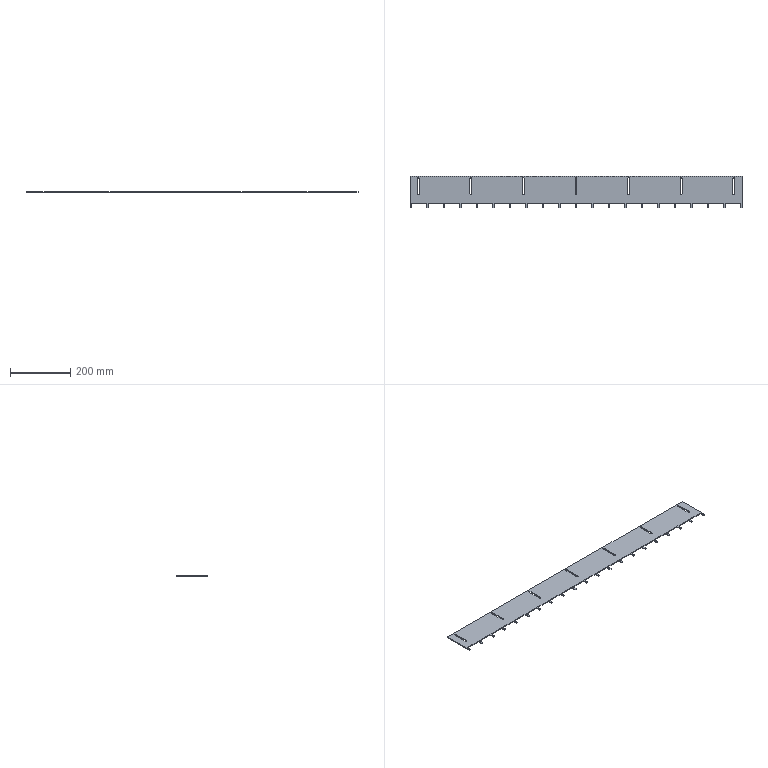Part | SolidWorks | features FlatPattern 1, HoleWzd 1, ICE 1, LPattern 1, SMBaseFlange 1, SheetMetal 1 | 1 solid | 114 faces | box 1105 x 105 x 3 mm | volume 296430 mm3 | plane 100 | cylinder 14 | commonest cylinder face diameters 5.8 x14